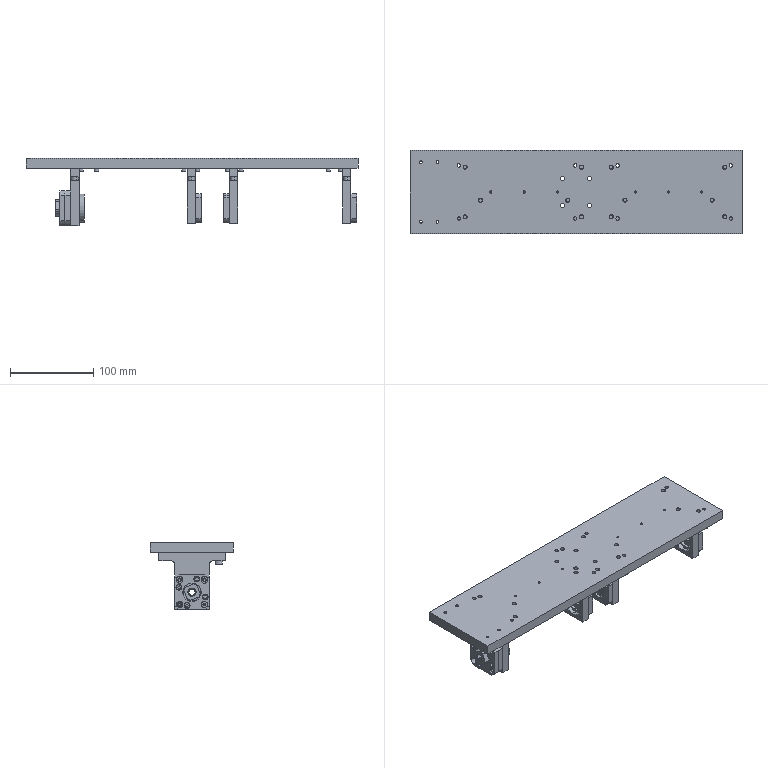Part | SolidWorks | features AEMSimFeature 1 | 34 solids | 829 faces | box 400 x 100 x 81 mm | volume 622322 mm3 | cylinder 387 | plane 330 | cone 86 | sphere 24 | spline 2 | commonest cylinder face diameters 5 x64 2.5 x36 3.4 x36 6.5 x24 5.5 x22 10 x21